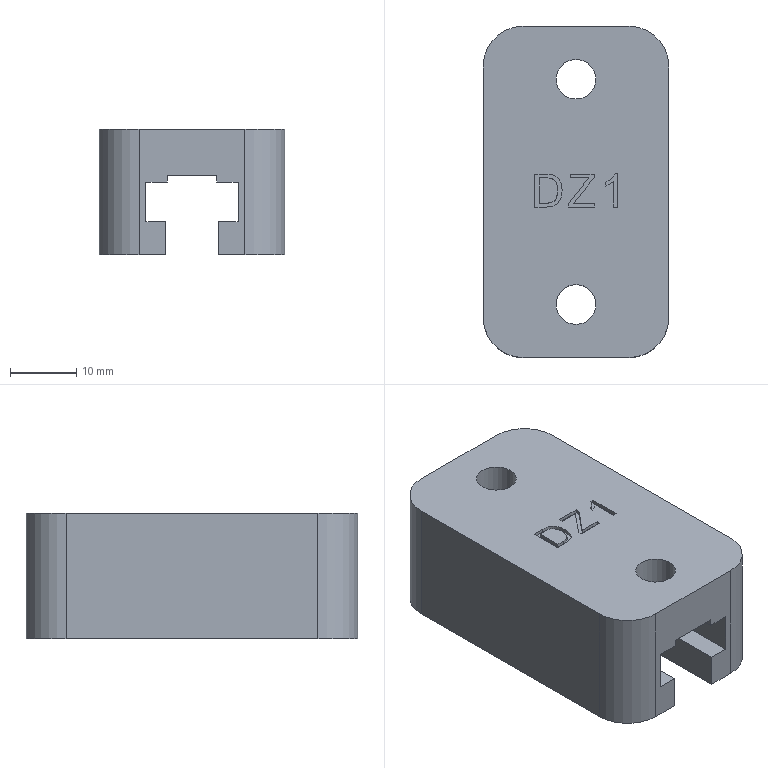Part | STEP file | solid 38 | 1 solid | 53 faces | box 27.996 x 50 x 19 mm | volume 19083 mm3 | plane 43 | cylinder 6 | other 4 | commonest cylinder face diameters 12 x4 6 x2